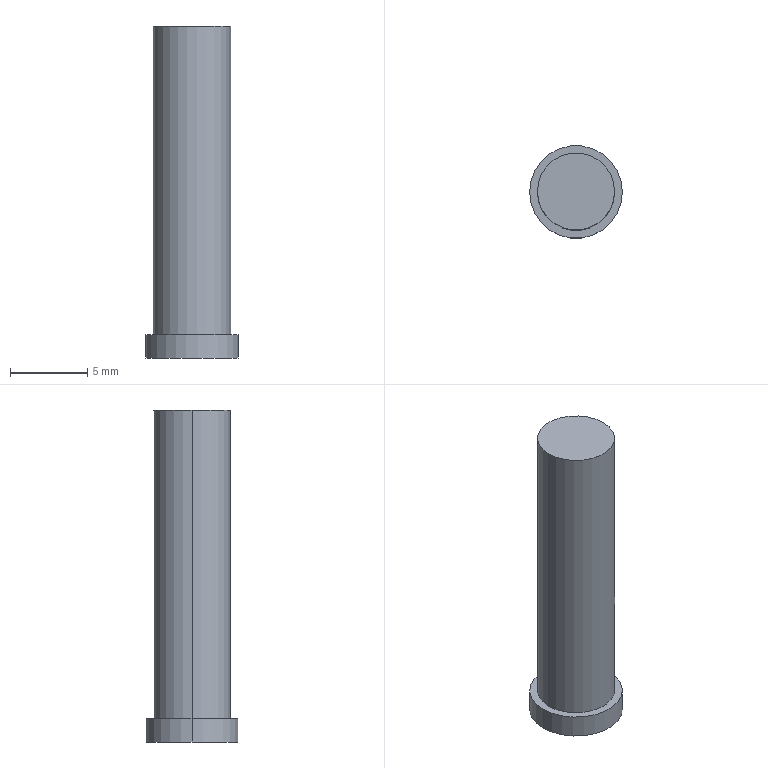Part | 1 solid | 7 faces | box 6 x 6 x 21.5 mm | volume 435.111 mm3 | cylinder 4 | plane 3 | commonest cylinder face diameters 5 x2 6 x2
STEP:
#1=CARTESIAN_POINT('',(0.,0.,0.));
#2=DIRECTION('',(0.,0.,1.));
#3=DIRECTION('',(1.,0.,0.));
#4=AXIS2_PLACEMENT_3D('',#1,#2,#3);
#5=CARTESIAN_POINT('',(2.5,0.,1.5));
#6=VERTEX_POINT('',#5);
#7=CARTESIAN_POINT('',(2.5,0.,21.5));
#8=VERTEX_POINT('',#7);
#9=CARTESIAN_POINT('',(2.5,0.,11.5));
#10=DIRECTION('',(0.,0.,1.));
#11=VECTOR('',#10,1.);
#12=LINE('',#9,#11);
#13=CARTESIAN_POINT('',(0.,0.,11.5));
#14=DIRECTION('',(0.,0.,1.));
#15=DIRECTION('',(1.,0.,0.));
#16=AXIS2_PLACEMENT_3D('',#13,#14,#15);
#17=CYLINDRICAL_SURFACE('',#16,2.5);
#18=CARTESIAN_POINT('',(0.,0.));
#19=DIRECTION('',(0.,1.));
#20=VECTOR('',#19,1.);
#21=LINE('',#18,#20);
#22=(GEOMETRIC_REPRESENTATION_CONTEXT(2)PARAMETRIC_REPRESENTATION_CONTEXT()REPRESENTATION_CONTEXT('',''));
#23=DEFINITIONAL_REPRESENTATION('',(#21),#22);
#24=PCURVE('',#17,#23);
#25=CARTESIAN_POINT('',(0.,0.,11.5));
#26=DIRECTION('',(0.,0.,1.));
#27=DIRECTION('',(1.,0.,0.));
#28=AXIS2_PLACEMENT_3D('',#25,#26,#27);
#29=CYLINDRICAL_SURFACE('',#28,2.5);
#30=CARTESIAN_POINT('',(6.283,0.));
#31=DIRECTION('',(0.,1.));
#32=VECTOR('',#31,1.);
#33=LINE('',#30,#32);
#34=(GEOMETRIC_REPRESENTATION_CONTEXT(2)PARAMETRIC_REPRESENTATION_CONTEXT()REPRESENTATION_CONTEXT('',''));
#35=DEFINITIONAL_REPRESENTATION('',(#33),#34);
#36=PCURVE('',#29,#35);
#37=SURFACE_CURVE('',#12,(#24,#36),.PCURVE_S1.);
#38=EDGE_CURVE('',#6,#8,#37,.T.);
#39=ORIENTED_EDGE('',*,*,#38,.F.);
#40=CARTESIAN_POINT('',(-2.5,0.,1.5));
#41=VERTEX_POINT('',#40);
#42=CARTESIAN_POINT('',(0.,0.,1.5));
#43=DIRECTION('',(0.,0.,1.));
#44=DIRECTION('',(1.,0.,0.));
#45=AXIS2_PLACEMENT_3D('',#42,#43,#44);
#46=CIRCLE('',#45,2.5);
#47=CARTESIAN_POINT('',(0.,-10.));
#48=DIRECTION('',(1.,0.));
#49=VECTOR('',#48,1.);
#50=LINE('',#47,#49);
#51=(GEOMETRIC_REPRESENTATION_CONTEXT(2)PARAMETRIC_REPRESENTATION_CONTEXT()REPRESENTATION_CONTEXT('',''));
#52=DEFINITIONAL_REPRESENTATION('',(#50),#51);
#53=PCURVE('',#17,#52);
#54=CARTESIAN_POINT('',(0.,0.,1.5));
#55=DIRECTION('',(0.,0.,1.));
#56=DIRECTION('',(1.,0.,0.));
#57=AXIS2_PLACEMENT_3D('',#54,#55,#56);
#58=PLANE('',#57);
#59=CARTESIAN_POINT('',(0.,0.));
#60=DIRECTION('',(1.,0.));
#61=AXIS2_PLACEMENT_2D('',#59,#60);
#62=CIRCLE('',#61,2.5);
#63=(GEOMETRIC_REPRESENTATION_CONTEXT(2)PARAMETRIC_REPRESENTATION_CONTEXT()REPRESENTATION_CONTEXT('',''));
#64=DEFINITIONAL_REPRESENTATION('',(#62),#63);
#65=PCURVE('',#58,#64);
#66=SURFACE_CURVE('',#46,(#53,#65),.PCURVE_S1.);
#67=EDGE_CURVE('',#6,#41,#66,.T.);
#68=ORIENTED_EDGE('',*,*,#67,.T.);
#69=CARTESIAN_POINT('',(-2.5,0.,21.5));
#70=VERTEX_POINT('',#69);
#71=CARTESIAN_POINT('',(-2.5,0.,11.5));
#72=DIRECTION('',(0.,0.,1.));
#73=VECTOR('',#72,1.);
#74=LINE('',#71,#73);
#75=CARTESIAN_POINT('',(3.142,0.));
#76=DIRECTION('',(0.,1.));
#77=VECTOR('',#76,1.);
#78=LINE('',#75,#77);
#79=(GEOMETRIC_REPRESENTATION_CONTEXT(2)PARAMETRIC_REPRESENTATION_CONTEXT()REPRESENTATION_CONTEXT('',''));
#80=DEFINITIONAL_REPRESENTATION('',(#78),#79);
#81=PCURVE('',#17,#80);
#82=CARTESIAN_POINT('',(3.142,0.));
#83=DIRECTION('',(0.,1.));
#84=VECTOR('',#83,1.);
#85=LINE('',#82,#84);
#86=(GEOMETRIC_REPRESENTATION_CONTEXT(2)PARAMETRIC_REPRESENTATION_CONTEXT()REPRESENTATION_CONTEXT('',''));
#87=DEFINITIONAL_REPRESENTATION('',(#85),#86);
#88=PCURVE('',#29,#87);
#89=SURFACE_CURVE('',#74,(#81,#88),.PCURVE_S1.);
#90=EDGE_CURVE('',#41,#70,#89,.T.);
#91=ORIENTED_EDGE('',*,*,#90,.T.);
#92=CARTESIAN_POINT('',(0.,0.,21.5));
#93=DIRECTION('',(0.,0.,1.));
#94=DIRECTION('',(1.,0.,0.));
#95=AXIS2_PLACEMENT_3D('',#92,#93,#94);
#96=CIRCLE('',#95,2.5);
#97=CARTESIAN_POINT('',(0.,10.));
#98=DIRECTION('',(1.,0.));
#99=VECTOR('',#98,1.);
#100=LINE('',#97,#99);
#101=(GEOMETRIC_REPRESENTATION_CONTEXT(2)PARAMETRIC_REPRESENTATION_CONTEXT()REPRESENTATION_CONTEXT('',''));
#102=DEFINITIONAL_REPRESENTATION('',(#100),#101);
#103=PCURVE('',#17,#102);
#104=CARTESIAN_POINT('',(0.,0.,21.5));
#105=DIRECTION('',(0.,0.,1.));
#106=DIRECTION('',(1.,0.,0.));
#107=AXIS2_PLACEMENT_3D('',#104,#105,#106);
#108=PLANE('',#107);
#109=CARTESIAN_POINT('',(0.,0.));
#110=DIRECTION('',(1.,0.));
#111=AXIS2_PLACEMENT_2D('',#109,#110);
#112=CIRCLE('',#111,2.5);
#113=(GEOMETRIC_REPRESENTATION_CONTEXT(2)PARAMETRIC_REPRESENTATION_CONTEXT()REPRESENTATION_CONTEXT('',''));
#114=DEFINITIONAL_REPRESENTATION('',(#112),#113);
#115=PCURVE('',#108,#114);
#116=SURFACE_CURVE('',#96,(#103,#115),.PCURVE_S1.);
#117=EDGE_CURVE('',#8,#70,#116,.T.);
#118=ORIENTED_EDGE('',*,*,#117,.F.);
#119=EDGE_LOOP('',(#39,#68,#91,#118));
#120=FACE_BOUND('',#119,.T.);
#121=ADVANCED_FACE('',(#120),#17,.T.);
#122=ORIENTED_EDGE('',*,*,#90,.F.);
#123=CARTESIAN_POINT('',(0.,0.,1.5));
#124=DIRECTION('',(0.,0.,1.));
#125=DIRECTION('',(1.,0.,0.));
#126=AXIS2_PLACEMENT_3D('',#123,#124,#125);
#127=CIRCLE('',#126,2.5);
#128=CARTESIAN_POINT('',(0.,-10.));
#129=DIRECTION('',(1.,0.));
#130=VECTOR('',#129,1.);
#131=LINE('',#128,#130);
#132=(GEOMETRIC_REPRESENTATION_CONTEXT(2)PARAMETRIC_REPRESENTATION_CONTEXT()REPRESENTATION_CONTEXT('',''));
#133=DEFINITIONAL_REPRESENTATION('',(#131),#132);
#134=PCURVE('',#29,#133);
#135=CARTESIAN_POINT('',(0.,0.));
#136=DIRECTION('',(1.,0.));
#137=AXIS2_PLACEMENT_2D('',#135,#136);
#138=CIRCLE('',#137,2.5);
#139=(GEOMETRIC_REPRESENTATION_CONTEXT(2)PARAMETRIC_REPRESENTATION_CONTEXT()REPRESENTATION_CONTEXT('',''));
#140=DEFINITIONAL_REPRESENTATION('',(#138),#139);
#141=PCURVE('',#58,#140);
#142=SURFACE_CURVE('',#127,(#134,#141),.PCURVE_S1.);
#143=EDGE_CURVE('',#41,#6,#142,.T.);
#144=ORIENTED_EDGE('',*,*,#143,.T.);
#145=ORIENTED_EDGE('',*,*,#38,.T.);
#146=CARTESIAN_POINT('',(0.,0.,21.5));
#147=DIRECTION('',(0.,0.,1.));
#148=DIRECTION('',(1.,0.,0.));
#149=AXIS2_PLACEMENT_3D('',#146,#147,#148);
#150=CIRCLE('',#149,2.5);
#151=CARTESIAN_POINT('',(0.,10.));
#152=DIRECTION('',(1.,0.));
#153=VECTOR('',#152,1.);
#154=LINE('',#151,#153);
#155=(GEOMETRIC_REPRESENTATION_CONTEXT(2)PARAMETRIC_REPRESENTATION_CONTEXT()REPRESENTATION_CONTEXT('',''));
#156=DEFINITIONAL_REPRESENTATION('',(#154),#155);
#157=PCURVE('',#29,#156);
#158=CARTESIAN_POINT('',(0.,0.));
#159=DIRECTION('',(1.,0.));
#160=AXIS2_PLACEMENT_2D('',#158,#159);
#161=CIRCLE('',#160,2.5);
#162=(GEOMETRIC_REPRESENTATION_CONTEXT(2)PARAMETRIC_REPRESENTATION_CONTEXT()REPRESENTATION_CONTEXT('',''));
#163=DEFINITIONAL_REPRESENTATION('',(#161),#162);
#164=PCURVE('',#108,#163);
#165=SURFACE_CURVE('',#150,(#157,#164),.PCURVE_S1.);
#166=EDGE_CURVE('',#70,#8,#165,.T.);
#167=ORIENTED_EDGE('',*,*,#166,.F.);
#168=EDGE_LOOP('',(#122,#144,#145,#167));
#169=FACE_BOUND('',#168,.T.);
#170=ADVANCED_FACE('',(#169),#29,.T.);
#171=ORIENTED_EDGE('',*,*,#117,.T.);
#172=ORIENTED_EDGE('',*,*,#166,.T.);
#173=EDGE_LOOP('',(#171,#172));
#174=FACE_BOUND('',#173,.T.);
#175=ADVANCED_FACE('',(#174),#108,.T.);
#176=CARTESIAN_POINT('',(3.,0.,1.5));
#177=VERTEX_POINT('',#176);
#178=CARTESIAN_POINT('',(-3.,0.,1.5));
#179=VERTEX_POINT('',#178);
#180=CARTESIAN_POINT('',(0.,0.,1.5));
#181=DIRECTION('',(0.,0.,1.));
#182=DIRECTION('',(1.,0.,0.));
#183=AXIS2_PLACEMENT_3D('',#180,#181,#182);
#184=CIRCLE('',#183,3.);
#185=CARTESIAN_POINT('',(0.,0.));
#186=DIRECTION('',(1.,0.));
#187=AXIS2_PLACEMENT_2D('',#185,#186);
#188=CIRCLE('',#187,3.);
#189=(GEOMETRIC_REPRESENTATION_CONTEXT(2)PARAMETRIC_REPRESENTATION_CONTEXT()REPRESENTATION_CONTEXT('',''));
#190=DEFINITIONAL_REPRESENTATION('',(#188),#189);
#191=PCURVE('',#58,#190);
#192=CARTESIAN_POINT('',(0.,0.,0.75));
#193=DIRECTION('',(0.,0.,1.));
#194=DIRECTION('',(1.,0.,0.));
#195=AXIS2_PLACEMENT_3D('',#192,#193,#194);
#196=CYLINDRICAL_SURFACE('',#195,3.);
#197=CARTESIAN_POINT('',(0.,0.75));
#198=DIRECTION('',(1.,0.));
#199=VECTOR('',#198,1.);
#200=LINE('',#197,#199);
#201=(GEOMETRIC_REPRESENTATION_CONTEXT(2)PARAMETRIC_REPRESENTATION_CONTEXT()REPRESENTATION_CONTEXT('',''));
#202=DEFINITIONAL_REPRESENTATION('',(#200),#201);
#203=PCURVE('',#196,#202);
#204=SURFACE_CURVE('',#184,(#191,#203),.PCURVE_S1.);
#205=EDGE_CURVE('',#177,#179,#204,.T.);
#206=ORIENTED_EDGE('',*,*,#205,.T.);
#207=CARTESIAN_POINT('',(0.,0.,1.5));
#208=DIRECTION('',(0.,0.,1.));
#209=DIRECTION('',(1.,0.,0.));
#210=AXIS2_PLACEMENT_3D('',#207,#208,#209);
#211=CIRCLE('',#210,3.);
#212=CARTESIAN_POINT('',(0.,0.));
#213=DIRECTION('',(1.,0.));
#214=AXIS2_PLACEMENT_2D('',#212,#213);
#215=CIRCLE('',#214,3.);
#216=(GEOMETRIC_REPRESENTATION_CONTEXT(2)PARAMETRIC_REPRESENTATION_CONTEXT()REPRESENTATION_CONTEXT('',''));
#217=DEFINITIONAL_REPRESENTATION('',(#215),#216);
#218=PCURVE('',#58,#217);
#219=CARTESIAN_POINT('',(0.,0.,0.75));
#220=DIRECTION('',(0.,0.,1.));
#221=DIRECTION('',(1.,0.,0.));
#222=AXIS2_PLACEMENT_3D('',#219,#220,#221);
#223=CYLINDRICAL_SURFACE('',#222,3.);
#224=CARTESIAN_POINT('',(0.,0.75));
#225=DIRECTION('',(1.,0.));
#226=VECTOR('',#225,1.);
#227=LINE('',#224,#226);
#228=(GEOMETRIC_REPRESENTATION_CONTEXT(2)PARAMETRIC_REPRESENTATION_CONTEXT()REPRESENTATION_CONTEXT('',''));
#229=DEFINITIONAL_REPRESENTATION('',(#227),#228);
#230=PCURVE('',#223,#229);
#231=SURFACE_CURVE('',#211,(#218,#230),.PCURVE_S1.);
#232=EDGE_CURVE('',#179,#177,#231,.T.);
#233=ORIENTED_EDGE('',*,*,#232,.T.);
#234=EDGE_LOOP('',(#206,#233));
#235=FACE_BOUND('',#234,.T.);
#236=ORIENTED_EDGE('',*,*,#67,.F.);
#237=ORIENTED_EDGE('',*,*,#143,.F.);
#238=EDGE_LOOP('',(#236,#237));
#239=FACE_BOUND('',#238,.T.);
#240=ADVANCED_FACE('',(#235,#239),#58,.T.);
#241=CARTESIAN_POINT('',(-3.,0.,0.));
#242=VERTEX_POINT('',#241);
#243=CARTESIAN_POINT('',(3.,0.,0.));
#244=VERTEX_POINT('',#243);
#245=CARTESIAN_POINT('',(0.,0.,0.));
#246=DIRECTION('',(0.,0.,1.));
#247=DIRECTION('',(1.,0.,0.));
#248=AXIS2_PLACEMENT_3D('',#245,#246,#247);
#249=CIRCLE('',#248,3.);
#250=CARTESIAN_POINT('',(0.,0.,0.));
#251=DIRECTION('',(0.,0.,1.));
#252=DIRECTION('',(1.,0.,0.));
#253=AXIS2_PLACEMENT_3D('',#250,#251,#252);
#254=PLANE('',#253);
#255=CARTESIAN_POINT('',(0.,0.));
#256=DIRECTION('',(1.,0.));
#257=AXIS2_PLACEMENT_2D('',#255,#256);
#258=CIRCLE('',#257,3.);
#259=(GEOMETRIC_REPRESENTATION_CONTEXT(2)PARAMETRIC_REPRESENTATION_CONTEXT()REPRESENTATION_CONTEXT('',''));
#260=DEFINITIONAL_REPRESENTATION('',(#258),#259);
#261=PCURVE('',#254,#260);
#262=CARTESIAN_POINT('',(0.,-0.75));
#263=DIRECTION('',(1.,0.));
#264=VECTOR('',#263,1.);
#265=LINE('',#262,#264);
#266=(GEOMETRIC_REPRESENTATION_CONTEXT(2)PARAMETRIC_REPRESENTATION_CONTEXT()REPRESENTATION_CONTEXT('',''));
#267=DEFINITIONAL_REPRESENTATION('',(#265),#266);
#268=PCURVE('',#223,#267);
#269=SURFACE_CURVE('',#249,(#261,#268),.PCURVE_S1.);
#270=EDGE_CURVE('',#242,#244,#269,.T.);
#271=ORIENTED_EDGE('',*,*,#270,.F.);
#272=CARTESIAN_POINT('',(0.,0.,0.));
#273=DIRECTION('',(0.,0.,1.));
#274=DIRECTION('',(1.,0.,0.));
#275=AXIS2_PLACEMENT_3D('',#272,#273,#274);
#276=CIRCLE('',#275,3.);
#277=CARTESIAN_POINT('',(0.,0.));
#278=DIRECTION('',(1.,0.));
#279=AXIS2_PLACEMENT_2D('',#277,#278);
#280=CIRCLE('',#279,3.);
#281=(GEOMETRIC_REPRESENTATION_CONTEXT(2)PARAMETRIC_REPRESENTATION_CONTEXT()REPRESENTATION_CONTEXT('',''));
#282=DEFINITIONAL_REPRESENTATION('',(#280),#281);
#283=PCURVE('',#254,#282);
#284=CARTESIAN_POINT('',(0.,-0.75));
#285=DIRECTION('',(1.,0.));
#286=VECTOR('',#285,1.);
#287=LINE('',#284,#286);
#288=(GEOMETRIC_REPRESENTATION_CONTEXT(2)PARAMETRIC_REPRESENTATION_CONTEXT()REPRESENTATION_CONTEXT('',''));
#289=DEFINITIONAL_REPRESENTATION('',(#287),#288);
#290=PCURVE('',#196,#289);
#291=SURFACE_CURVE('',#276,(#283,#290),.PCURVE_S1.);
#292=EDGE_CURVE('',#244,#242,#291,.T.);
#293=ORIENTED_EDGE('',*,*,#292,.F.);
#294=EDGE_LOOP('',(#271,#293));
#295=FACE_BOUND('',#294,.T.);
#296=ADVANCED_FACE('',(#295),#254,.F.);
#297=CARTESIAN_POINT('',(-3.,0.,0.75));
#298=DIRECTION('',(0.,0.,1.));
#299=VECTOR('',#298,1.);
#300=LINE('',#297,#299);
#301=CARTESIAN_POINT('',(3.142,0.));
#302=DIRECTION('',(0.,1.));
#303=VECTOR('',#302,1.);
#304=LINE('',#301,#303);
#305=(GEOMETRIC_REPRESENTATION_CONTEXT(2)PARAMETRIC_REPRESENTATION_CONTEXT()REPRESENTATION_CONTEXT('',''));
#306=DEFINITIONAL_REPRESENTATION('',(#304),#305);
#307=PCURVE('',#223,#306);
#308=CARTESIAN_POINT('',(3.142,0.));
#309=DIRECTION('',(0.,1.));
#310=VECTOR('',#309,1.);
#311=LINE('',#308,#310);
#312=(GEOMETRIC_REPRESENTATION_CONTEXT(2)PARAMETRIC_REPRESENTATION_CONTEXT()REPRESENTATION_CONTEXT('',''));
#313=DEFINITIONAL_REPRESENTATION('',(#311),#312);
#314=PCURVE('',#196,#313);
#315=SURFACE_CURVE('',#300,(#307,#314),.PCURVE_S1.);
#316=EDGE_CURVE('',#242,#179,#315,.T.);
#317=ORIENTED_EDGE('',*,*,#316,.F.);
#318=ORIENTED_EDGE('',*,*,#270,.T.);
#319=CARTESIAN_POINT('',(3.,0.,0.75));
#320=DIRECTION('',(0.,0.,1.));
#321=VECTOR('',#320,1.);
#322=LINE('',#319,#321);
#323=CARTESIAN_POINT('',(6.283,0.));
#324=DIRECTION('',(0.,1.));
#325=VECTOR('',#324,1.);
#326=LINE('',#323,#325);
#327=(GEOMETRIC_REPRESENTATION_CONTEXT(2)PARAMETRIC_REPRESENTATION_CONTEXT()REPRESENTATION_CONTEXT('',''));
#328=DEFINITIONAL_REPRESENTATION('',(#326),#327);
#329=PCURVE('',#223,#328);
#330=CARTESIAN_POINT('',(0.,0.));
#331=DIRECTION('',(0.,1.));
#332=VECTOR('',#331,1.);
#333=LINE('',#330,#332);
#334=(GEOMETRIC_REPRESENTATION_CONTEXT(2)PARAMETRIC_REPRESENTATION_CONTEXT()REPRESENTATION_CONTEXT('',''));
#335=DEFINITIONAL_REPRESENTATION('',(#333),#334);
#336=PCURVE('',#196,#335);
#337=SURFACE_CURVE('',#322,(#329,#336),.PCURVE_S1.);
#338=EDGE_CURVE('',#244,#177,#337,.T.);
#339=ORIENTED_EDGE('',*,*,#338,.T.);
#340=ORIENTED_EDGE('',*,*,#232,.F.);
#341=EDGE_LOOP('',(#317,#318,#339,#340));
#342=FACE_BOUND('',#341,.T.);
#343=ADVANCED_FACE('',(#342),#223,.T.);
#344=ORIENTED_EDGE('',*,*,#338,.F.);
#345=ORIENTED_EDGE('',*,*,#292,.T.);
#346=ORIENTED_EDGE('',*,*,#316,.T.);
#347=ORIENTED_EDGE('',*,*,#205,.F.);
#348=EDGE_LOOP('',(#344,#345,#346,#347));
#349=FACE_BOUND('',#348,.T.);
#350=ADVANCED_FACE('',(#349),#196,.T.);
#351=CLOSED_SHELL('',(#121,#170,#175,#240,#296,#343,#350));
#352=MANIFOLD_SOLID_BREP('',#351);
#353=(LENGTH_UNIT()NAMED_UNIT(*)SI_UNIT(.MILLI.,.METRE.));
#354=UNCERTAINTY_MEASURE_WITH_UNIT(LENGTH_MEASURE(0.0000001),#353,'','');
#355=(NAMED_UNIT(*)PLANE_ANGLE_UNIT()SI_UNIT($,.RADIAN.));
#356=(NAMED_UNIT(*)SI_UNIT($,.STERADIAN.)SOLID_ANGLE_UNIT());
#357=(GEOMETRIC_REPRESENTATION_CONTEXT(3)GLOBAL_UNCERTAINTY_ASSIGNED_CONTEXT((#354))GLOBAL_UNIT_ASSIGNED_CONTEXT((#353,#355,#356))REPRESENTATION_CONTEXT('',''));
#358=ADVANCED_BREP_SHAPE_REPRESENTATION('',(#4,#352),#357);